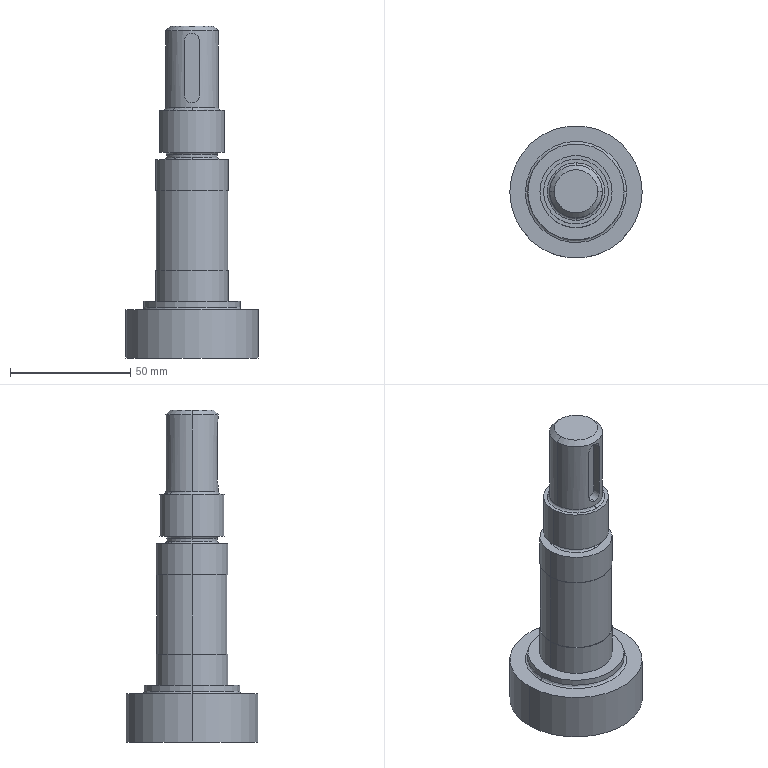Part | SolidWorks | features BaseBody 1 | 1 solid | 65 faces | box 55 x 55 x 138 mm | volume 113601 mm3 | cylinder 31 | cone 14 | plane 12 | torus 6 | spline 2 | commonest cylinder face diameters 6.8 x8 8 x4 30 x4 6 x3 21 x2 22 x2